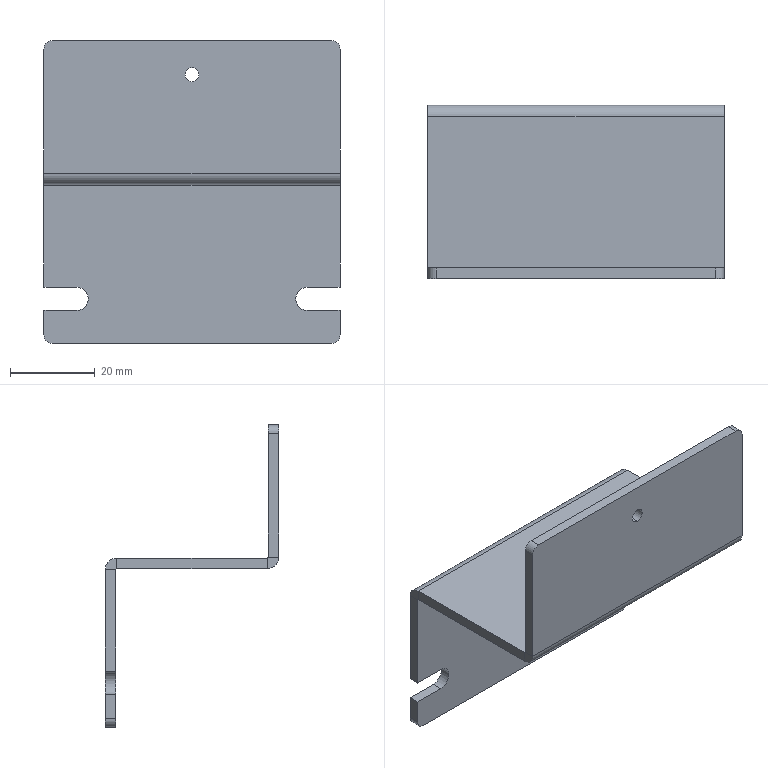Part | STEP file | 1 solid | 36 faces | box 70 x 41 x 71.5 mm | volume 18730 mm3 | plane 24 | cylinder 12 | commonest cylinder face diameters 4 x4 0.4 x2 3.3 x2 5.4 x2 5.5 x2